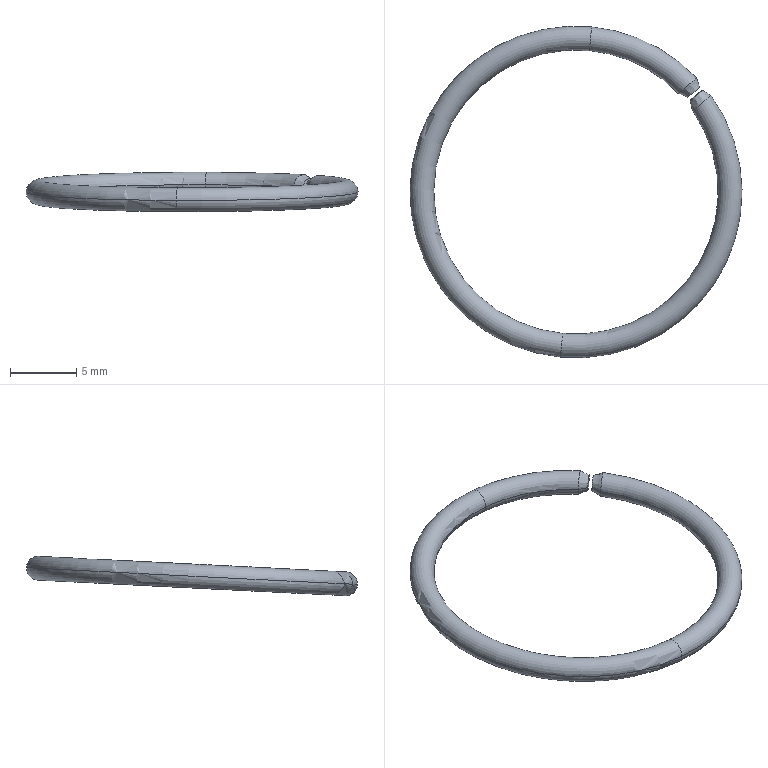Part | SolidWorks | features BaseBody 1 | 1 solid | 12 faces | box 25.1 x 25.07 x 2.979 mm | volume 184.393 mm3 | torus 6 | spline 4 | plane 2
STEP:
#1=CARTESIAN_POINT('',(1925.446,-674.153,857.254));
#2=VERTEX_POINT('',#1);
#3=CARTESIAN_POINT('',(1932.144,-677.358,857.099));
#4=VERTEX_POINT('',#3);
#5=CARTESIAN_POINT('',(1924.436,-684.842,856.711));
#6=DIRECTION('',(0.001134,0.05057,-0.9987));
#7=DIRECTION('',(0.9956,-0.09388,-0.003624));
#8=AXIS2_PLACEMENT_3D('',#5,#6,#7);
#9=CIRCLE('',#8,10.75);
#10=EDGE_CURVE('',#2,#4,#9,.T.);
#11=ORIENTED_EDGE('',*,*,#10,.F.);
#12=CARTESIAN_POINT('',(1925.615,-672.363,857.345));
#13=VERTEX_POINT('',#12);
#14=CARTESIAN_POINT('',(1925.531,-673.258,857.299));
#15=DIRECTION('',(0.9956,-0.09388,-0.003624));
#16=DIRECTION('',(0.09388,0.9956,0.));
#17=AXIS2_PLACEMENT_3D('',#14,#15,#16);
#18=CIRCLE('',#17,0.9);
#19=EDGE_CURVE('',#2,#13,#18,.T.);
#20=ORIENTED_EDGE('',*,*,#19,.T.);
#21=CARTESIAN_POINT('',(1933.534,-676.209,857.159));
#22=VERTEX_POINT('',#21);
#23=CARTESIAN_POINT('',(1924.436,-684.842,856.711));
#24=DIRECTION('',(-0.001134,-0.05057,0.9987));
#25=DIRECTION('',(0.9956,-0.09388,-0.003624));
#26=AXIS2_PLACEMENT_3D('',#23,#24,#25);
#27=CIRCLE('',#26,12.55);
#28=EDGE_CURVE('',#22,#13,#27,.T.);
#29=ORIENTED_EDGE('',*,*,#28,.F.);
#30=CARTESIAN_POINT('',(1932.144,-677.358,857.099));
#31=CARTESIAN_POINT('',(1932.144,-677.352,856.98));
#32=CARTESIAN_POINT('',(1932.162,-677.332,856.866));
#33=CARTESIAN_POINT('',(1932.232,-677.262,856.65));
#34=CARTESIAN_POINT('',(1932.283,-677.215,856.553));
#35=CARTESIAN_POINT('',(1932.411,-677.098,856.392));
#36=CARTESIAN_POINT('',(1932.488,-677.03,856.329));
#37=CARTESIAN_POINT('',(1932.657,-676.889,856.246));
#38=CARTESIAN_POINT('',(1932.748,-676.812,856.226));
#39=CARTESIAN_POINT('',(1932.928,-676.662,856.234));
#40=CARTESIAN_POINT('',(1933.02,-676.588,856.261));
#41=CARTESIAN_POINT('',(1933.187,-676.453,856.358));
#42=CARTESIAN_POINT('',(1933.264,-676.392,856.428));
#43=CARTESIAN_POINT('',(1933.459,-676.247,856.685));
#44=CARTESIAN_POINT('',(1933.534,-676.197,856.921));
#45=CARTESIAN_POINT('',(1933.534,-676.209,857.159));
#46=B_SPLINE_CURVE_WITH_KNOTS('',3,(#30,#31,#32,#33,#34,#35,#36,#37,#38,#39,#40,#41,#42,#43,#44,#45),.UNSPECIFIED.,.F.,.F.,(4,2,2,2,2,2,2,4),(0.,0.0003506,0.0007011,0.001052,0.001402,0.001753,0.002103,0.002805),.UNSPECIFIED.);
#47=EDGE_CURVE('',#4,#22,#46,.T.);
#48=ORIENTED_EDGE('',*,*,#47,.F.);
#49=EDGE_LOOP('',(#11,#20,#29,#48));
#50=FACE_OUTER_BOUND('',#49,.T.);
#51=CARTESIAN_POINT('',(1924.436,-684.842,856.711));
#52=DIRECTION('',(-0.001134,-0.05057,0.9987));
#53=DIRECTION('',(-0.09394,-0.9943,-0.05046));
#54=AXIS2_PLACEMENT_3D('',#51,#52,#53);
#55=TOROIDAL_SURFACE('',#54,11.65,0.9);
#56=ADVANCED_FACE('',(#50),#55,.T.);
#57=ORIENTED_EDGE('',*,*,#19,.F.);
#58=CARTESIAN_POINT('',(1923.426,-695.531,856.169));
#59=VERTEX_POINT('',#58);
#60=CARTESIAN_POINT('',(1924.436,-684.842,856.711));
#61=DIRECTION('',(0.001134,0.05057,-0.9987));
#62=DIRECTION('',(0.9956,-0.09388,-0.003624));
#63=AXIS2_PLACEMENT_3D('',#60,#61,#62);
#64=CIRCLE('',#63,10.75);
#65=EDGE_CURVE('',#59,#2,#64,.T.);
#66=ORIENTED_EDGE('',*,*,#65,.F.);
#67=CARTESIAN_POINT('',(1923.257,-697.32,856.078));
#68=VERTEX_POINT('',#67);
#69=CARTESIAN_POINT('',(1923.342,-696.425,856.124));
#70=DIRECTION('',(-0.9956,0.09388,0.003624));
#71=DIRECTION('',(-0.09388,-0.9956,0.));
#72=AXIS2_PLACEMENT_3D('',#69,#70,#71);
#73=CIRCLE('',#72,0.9);
#74=EDGE_CURVE('',#59,#68,#73,.T.);
#75=ORIENTED_EDGE('',*,*,#74,.T.);
#76=CARTESIAN_POINT('',(1924.436,-684.842,856.711));
#77=DIRECTION('',(-0.001134,-0.05057,0.9987));
#78=DIRECTION('',(0.9956,-0.09388,-0.003624));
#79=AXIS2_PLACEMENT_3D('',#76,#77,#78);
#80=CIRCLE('',#79,12.55);
#81=EDGE_CURVE('',#13,#68,#80,.T.);
#82=ORIENTED_EDGE('',*,*,#81,.F.);
#83=EDGE_LOOP('',(#57,#66,#75,#82));
#84=FACE_OUTER_BOUND('',#83,.T.);
#85=CARTESIAN_POINT('',(1924.436,-684.842,856.711));
#86=DIRECTION('',(-0.001134,-0.05057,0.9987));
#87=DIRECTION('',(-0.09394,-0.9943,-0.05046));
#88=AXIS2_PLACEMENT_3D('',#85,#86,#87);
#89=TOROIDAL_SURFACE('',#88,11.65,0.9);
#90=ADVANCED_FACE('',(#84),#89,.T.);
#91=ORIENTED_EDGE('',*,*,#28,.T.);
#92=CARTESIAN_POINT('',(1925.531,-673.258,857.299));
#93=DIRECTION('',(0.9956,-0.09388,-0.003624));
#94=DIRECTION('',(0.09388,0.9956,0.));
#95=AXIS2_PLACEMENT_3D('',#92,#93,#94);
#96=CIRCLE('',#95,0.9);
#97=EDGE_CURVE('',#13,#2,#96,.T.);
#98=ORIENTED_EDGE('',*,*,#97,.T.);
#99=ORIENTED_EDGE('',*,*,#10,.T.);
#100=CARTESIAN_POINT('',(1933.534,-676.209,857.159));
#101=CARTESIAN_POINT('',(1933.534,-676.215,857.278));
#102=CARTESIAN_POINT('',(1933.516,-676.235,857.392));
#103=CARTESIAN_POINT('',(1933.446,-676.304,857.608));
#104=CARTESIAN_POINT('',(1933.394,-676.351,857.705));
#105=CARTESIAN_POINT('',(1933.263,-676.464,857.866));
#106=CARTESIAN_POINT('',(1933.187,-676.532,857.93));
#107=CARTESIAN_POINT('',(1933.02,-676.676,858.012));
#108=CARTESIAN_POINT('',(1932.928,-676.752,858.032));
#109=CARTESIAN_POINT('',(1932.747,-676.902,858.024));
#110=CARTESIAN_POINT('',(1932.656,-676.976,857.997));
#111=CARTESIAN_POINT('',(1932.487,-677.109,857.9));
#112=CARTESIAN_POINT('',(1932.41,-677.17,857.831));
#113=CARTESIAN_POINT('',(1932.219,-677.32,857.573));
#114=CARTESIAN_POINT('',(1932.144,-677.37,857.337));
#115=CARTESIAN_POINT('',(1932.144,-677.358,857.099));
#116=B_SPLINE_CURVE_WITH_KNOTS('',3,(#100,#101,#102,#103,#104,#105,#106,#107,#108,#109,#110,#111,#112,#113,#114,#115),.UNSPECIFIED.,.F.,.F.,(4,2,2,2,2,2,2,4),(0.,0.0003506,0.0007012,0.001052,0.001402,0.001753,0.002104,0.002805),.UNSPECIFIED.);
#117=EDGE_CURVE('',#22,#4,#116,.T.);
#118=ORIENTED_EDGE('',*,*,#117,.F.);
#119=EDGE_LOOP('',(#91,#98,#99,#118));
#120=FACE_OUTER_BOUND('',#119,.T.);
#121=CARTESIAN_POINT('',(1924.436,-684.842,856.711));
#122=DIRECTION('',(-0.001134,-0.05057,0.9987));
#123=DIRECTION('',(-0.09394,-0.9943,-0.05046));
#124=AXIS2_PLACEMENT_3D('',#121,#122,#123);
#125=TOROIDAL_SURFACE('',#124,11.65,0.9);
#126=ADVANCED_FACE('',(#120),#125,.T.);
#127=ORIENTED_EDGE('',*,*,#97,.F.);
#128=ORIENTED_EDGE('',*,*,#81,.T.);
#129=CARTESIAN_POINT('',(1923.342,-696.425,856.124));
#130=DIRECTION('',(-0.9956,0.09388,0.003624));
#131=DIRECTION('',(-0.09388,-0.9956,0.));
#132=AXIS2_PLACEMENT_3D('',#129,#130,#131);
#133=CIRCLE('',#132,0.9);
#134=EDGE_CURVE('',#68,#59,#133,.T.);
#135=ORIENTED_EDGE('',*,*,#134,.T.);
#136=ORIENTED_EDGE('',*,*,#65,.T.);
#137=EDGE_LOOP('',(#127,#128,#135,#136));
#138=FACE_OUTER_BOUND('',#137,.T.);
#139=CARTESIAN_POINT('',(1924.436,-684.842,856.711));
#140=DIRECTION('',(-0.001134,-0.05057,0.9987));
#141=DIRECTION('',(-0.09394,-0.9943,-0.05046));
#142=AXIS2_PLACEMENT_3D('',#139,#140,#141);
#143=TOROIDAL_SURFACE('',#142,11.65,0.9);
#144=ADVANCED_FACE('',(#138),#143,.T.);
#145=ORIENTED_EDGE('',*,*,#134,.F.);
#146=CARTESIAN_POINT('',(1934.63,-677.531,857.093));
#147=VERTEX_POINT('',#146);
#148=CARTESIAN_POINT('',(1924.436,-684.842,856.711));
#149=DIRECTION('',(-0.001134,-0.05057,0.9987));
#150=DIRECTION('',(0.9956,-0.09388,-0.003624));
#151=AXIS2_PLACEMENT_3D('',#148,#149,#150);
#152=CIRCLE('',#151,12.55);
#153=EDGE_CURVE('',#68,#147,#152,.T.);
#154=ORIENTED_EDGE('',*,*,#153,.T.);
#155=CARTESIAN_POINT('',(1933.239,-678.68,857.033));
#156=VERTEX_POINT('',#155);
#157=CARTESIAN_POINT('',(1933.239,-678.68,857.033));
#158=CARTESIAN_POINT('',(1933.239,-678.686,857.152));
#159=CARTESIAN_POINT('',(1933.257,-678.678,857.268));
#160=CARTESIAN_POINT('',(1933.327,-678.631,857.49));
#161=CARTESIAN_POINT('',(1933.378,-678.594,857.592));
#162=CARTESIAN_POINT('',(1933.509,-678.498,857.764));
#163=CARTESIAN_POINT('',(1933.586,-678.437,857.834));
#164=CARTESIAN_POINT('',(1933.752,-678.302,857.931));
#165=CARTESIAN_POINT('',(1933.844,-678.228,857.958));
#166=CARTESIAN_POINT('',(1934.025,-678.079,857.966));
#167=CARTESIAN_POINT('',(1934.116,-678.001,857.947));
#168=CARTESIAN_POINT('',(1934.284,-677.859,857.864));
#169=CARTESIAN_POINT('',(1934.362,-677.792,857.801));
#170=CARTESIAN_POINT('',(1934.554,-677.618,857.56));
#171=CARTESIAN_POINT('',(1934.63,-677.544,857.331));
#172=CARTESIAN_POINT('',(1934.63,-677.531,857.093));
#173=B_SPLINE_CURVE_WITH_KNOTS('',3,(#157,#158,#159,#160,#161,#162,#163,#164,#165,#166,#167,#168,#169,#170,#171,#172),.UNSPECIFIED.,.F.,.F.,(4,2,2,2,2,2,2,4),(0.,0.0003506,0.0007011,0.001052,0.001402,0.001753,0.002103,0.002805),.UNSPECIFIED.);
#174=EDGE_CURVE('',#156,#147,#173,.T.);
#175=ORIENTED_EDGE('',*,*,#174,.F.);
#176=CARTESIAN_POINT('',(1924.436,-684.842,856.711));
#177=DIRECTION('',(0.001134,0.05057,-0.9987));
#178=DIRECTION('',(0.9956,-0.09388,-0.003624));
#179=AXIS2_PLACEMENT_3D('',#176,#177,#178);
#180=CIRCLE('',#179,10.75);
#181=EDGE_CURVE('',#156,#59,#180,.T.);
#182=ORIENTED_EDGE('',*,*,#181,.T.);
#183=EDGE_LOOP('',(#145,#154,#175,#182));
#184=FACE_OUTER_BOUND('',#183,.T.);
#185=CARTESIAN_POINT('',(1924.436,-684.842,856.711));
#186=DIRECTION('',(-0.001134,-0.05057,0.9987));
#187=DIRECTION('',(-0.09394,-0.9943,-0.05046));
#188=AXIS2_PLACEMENT_3D('',#185,#186,#187);
#189=TOROIDAL_SURFACE('',#188,11.65,0.9);
#190=ADVANCED_FACE('',(#184),#189,.T.);
#191=ORIENTED_EDGE('',*,*,#74,.F.);
#192=ORIENTED_EDGE('',*,*,#181,.F.);
#193=CARTESIAN_POINT('',(1934.63,-677.531,857.093));
#194=CARTESIAN_POINT('',(1934.63,-677.525,856.974));
#195=CARTESIAN_POINT('',(1934.613,-677.534,856.859));
#196=CARTESIAN_POINT('',(1934.543,-677.581,856.636));
#197=CARTESIAN_POINT('',(1934.492,-677.619,856.535));
#198=CARTESIAN_POINT('',(1934.365,-677.719,856.363));
#199=CARTESIAN_POINT('',(1934.287,-677.779,856.293));
#200=CARTESIAN_POINT('',(1934.119,-677.912,856.196));
#201=CARTESIAN_POINT('',(1934.028,-677.987,856.168));
#202=CARTESIAN_POINT('',(1933.847,-678.136,856.16));
#203=CARTESIAN_POINT('',(1933.755,-678.213,856.18));
#204=CARTESIAN_POINT('',(1933.589,-678.357,856.262));
#205=CARTESIAN_POINT('',(1933.511,-678.424,856.325));
#206=CARTESIAN_POINT('',(1933.315,-678.594,856.566));
#207=CARTESIAN_POINT('',(1933.24,-678.668,856.795));
#208=CARTESIAN_POINT('',(1933.239,-678.68,857.033));
#209=B_SPLINE_CURVE_WITH_KNOTS('',3,(#193,#194,#195,#196,#197,#198,#199,#200,#201,#202,#203,#204,#205,#206,#207,#208),.UNSPECIFIED.,.F.,.F.,(4,2,2,2,2,2,2,4),(0.,0.0003506,0.0007012,0.001052,0.001402,0.001753,0.002104,0.002805),.UNSPECIFIED.);
#210=EDGE_CURVE('',#147,#156,#209,.T.);
#211=ORIENTED_EDGE('',*,*,#210,.F.);
#212=ORIENTED_EDGE('',*,*,#153,.F.);
#213=EDGE_LOOP('',(#191,#192,#211,#212));
#214=FACE_OUTER_BOUND('',#213,.T.);
#215=CARTESIAN_POINT('',(1924.436,-684.842,856.711));
#216=DIRECTION('',(-0.001134,-0.05057,0.9987));
#217=DIRECTION('',(-0.09394,-0.9943,-0.05046));
#218=AXIS2_PLACEMENT_3D('',#215,#216,#217);
#219=TOROIDAL_SURFACE('',#218,11.65,0.9);
#220=ADVANCED_FACE('',(#214),#219,.T.);
#221=CARTESIAN_POINT('',(1933.785,-676.906,857.124));
#222=VERTEX_POINT('',#221);
#223=CARTESIAN_POINT('',(1933.534,-676.209,857.159));
#224=DIRECTION('',(-0.3381,0.9399,0.04721));
#225=VECTOR('',#224,1000.);
#226=LINE('',#223,#225);
#227=EDGE_CURVE('',#222,#22,#226,.T.);
#228=ORIENTED_EDGE('',*,*,#227,.F.);
#229=CARTESIAN_POINT('',(1932.863,-677.669,857.084));
#230=VERTEX_POINT('',#229);
#231=CARTESIAN_POINT('',(1932.863,-677.669,857.084));
#232=CARTESIAN_POINT('',(1932.863,-677.667,857.045));
#233=CARTESIAN_POINT('',(1932.872,-677.653,856.927));
#234=CARTESIAN_POINT('',(1932.942,-677.584,856.707));
#235=CARTESIAN_POINT('',(1933.146,-677.405,856.498));
#236=CARTESIAN_POINT('',(1933.454,-677.149,856.488));
#237=CARTESIAN_POINT('',(1933.688,-676.966,856.702));
#238=CARTESIAN_POINT('',(1933.774,-676.907,856.948));
#239=CARTESIAN_POINT('',(1933.785,-676.904,857.08));
#240=CARTESIAN_POINT('',(1933.785,-676.906,857.124));
#241=B_SPLINE_CURVE_WITH_KNOTS('',3,(#231,#232,#233,#234,#235,#236,#237,#238,#239,#240),.UNSPECIFIED.,.F.,.F.,(4,1,1,1,1,1,1,4),(0.,0.06667,0.2,0.4,0.6,0.8,0.9333,1.),.UNSPECIFIED.);
#242=EDGE_CURVE('',#230,#222,#241,.T.);
#243=ORIENTED_EDGE('',*,*,#242,.F.);
#244=CARTESIAN_POINT('',(1932.144,-677.358,857.099));
#245=DIRECTION('',(0.918,-0.3961,-0.01902));
#246=VECTOR('',#245,1000.);
#247=LINE('',#244,#246);
#248=EDGE_CURVE('',#4,#230,#247,.T.);
#249=ORIENTED_EDGE('',*,*,#248,.F.);
#250=ORIENTED_EDGE('',*,*,#47,.T.);
#251=EDGE_LOOP('',(#228,#243,#249,#250));
#252=FACE_OUTER_BOUND('',#251,.T.);
#253=CARTESIAN_POINT('',(1932.103,-677.341,857.17));
#254=CARTESIAN_POINT('',(1932.37,-677.457,857.154));
#255=CARTESIAN_POINT('',(1932.638,-677.572,857.138));
#256=CARTESIAN_POINT('',(1932.905,-677.687,857.123));
#257=CARTESIAN_POINT('',(1932.101,-677.341,857.146));
#258=CARTESIAN_POINT('',(1932.369,-677.457,857.134));
#259=CARTESIAN_POINT('',(1932.637,-677.572,857.122));
#260=CARTESIAN_POINT('',(1932.905,-677.687,857.11));
#261=CARTESIAN_POINT('',(1932.099,-677.339,857.056));
#262=CARTESIAN_POINT('',(1932.367,-677.455,857.057));
#263=CARTESIAN_POINT('',(1932.635,-677.57,857.058));
#264=CARTESIAN_POINT('',(1932.903,-677.686,857.059));
#265=CARTESIAN_POINT('',(1932.118,-677.312,856.833));
#266=CARTESIAN_POINT('',(1932.383,-677.432,856.866));
#267=CARTESIAN_POINT('',(1932.648,-677.552,856.899));
#268=CARTESIAN_POINT('',(1932.913,-677.672,856.932));
#269=CARTESIAN_POINT('',(1932.251,-677.182,856.47));
#270=CARTESIAN_POINT('',(1932.494,-677.324,856.553));
#271=CARTESIAN_POINT('',(1932.737,-677.465,856.636));
#272=CARTESIAN_POINT('',(1932.98,-677.606,856.719));
#273=CARTESIAN_POINT('',(1932.605,-676.873,856.178));
#274=CARTESIAN_POINT('',(1932.795,-677.06,856.29));
#275=CARTESIAN_POINT('',(1932.985,-677.247,856.403));
#276=CARTESIAN_POINT('',(1933.176,-677.434,856.515));
#277=CARTESIAN_POINT('',(1933.069,-676.491,856.224));
#278=CARTESIAN_POINT('',(1933.204,-676.722,856.317));
#279=CARTESIAN_POINT('',(1933.34,-676.954,856.409));
#280=CARTESIAN_POINT('',(1933.475,-677.185,856.502));
#281=CARTESIAN_POINT('',(1933.39,-676.243,856.56));
#282=CARTESIAN_POINT('',(1933.495,-676.497,856.61));
#283=CARTESIAN_POINT('',(1933.599,-676.751,856.659));
#284=CARTESIAN_POINT('',(1933.704,-677.005,856.709));
#285=CARTESIAN_POINT('',(1933.505,-676.166,856.912));
#286=CARTESIAN_POINT('',(1933.599,-676.426,856.925));
#287=CARTESIAN_POINT('',(1933.694,-676.687,856.937));
#288=CARTESIAN_POINT('',(1933.789,-676.947,856.95));
#289=CARTESIAN_POINT('',(1933.521,-676.163,857.121));
#290=CARTESIAN_POINT('',(1933.614,-676.424,857.112));
#291=CARTESIAN_POINT('',(1933.708,-676.684,857.103));
#292=CARTESIAN_POINT('',(1933.801,-676.944,857.094));
#293=CARTESIAN_POINT('',(1933.518,-676.169,857.204));
#294=CARTESIAN_POINT('',(1933.612,-676.429,857.186));
#295=CARTESIAN_POINT('',(1933.706,-676.689,857.169));
#296=CARTESIAN_POINT('',(1933.799,-676.948,857.152));
#297=CARTESIAN_POINT('',(1933.517,-676.171,857.225));
#298=CARTESIAN_POINT('',(1933.611,-676.431,857.206));
#299=CARTESIAN_POINT('',(1933.705,-676.69,857.186));
#300=CARTESIAN_POINT('',(1933.798,-676.95,857.166));
#301=B_SPLINE_SURFACE_WITH_KNOTS('',3,3,((#253,#254,#255,#256),(#257,#258,#259,#260),(#261,#262,#263,#264),(#265,#266,#267,#268),(#269,#270,#271,#272),(#273,#274,#275,#276),(#277,#278,#279,#280),(#281,#282,#283,#284),(#285,#286,#287,#288),(#289,#290,#291,#292),(#293,#294,#295,#296),(#297,#298,#299,#300)),.UNSPECIFIED.,.F.,.F.,.F.,(4,1,1,1,1,1,1,1,1,4),(4,4),(0.,0.02206,0.08578,0.2132,0.4044,0.5956,0.7868,0.9142,0.9779,1.),(0.,1.),.UNSPECIFIED.);
#302=ADVANCED_FACE('',(#252),#301,.T.);
#303=ORIENTED_EDGE('',*,*,#248,.T.);
#304=CARTESIAN_POINT('',(1933.785,-676.906,857.124));
#305=CARTESIAN_POINT('',(1933.785,-676.909,857.168));
#306=CARTESIAN_POINT('',(1933.774,-676.925,857.299));
#307=CARTESIAN_POINT('',(1933.687,-677.008,857.538));
#308=CARTESIAN_POINT('',(1933.452,-677.212,857.732));
#309=CARTESIAN_POINT('',(1933.145,-677.465,857.695));
#310=CARTESIAN_POINT('',(1932.941,-677.623,857.469));
#311=CARTESIAN_POINT('',(1932.872,-677.669,857.242));
#312=CARTESIAN_POINT('',(1932.863,-677.671,857.124));
#313=CARTESIAN_POINT('',(1932.863,-677.669,857.084));
#314=B_SPLINE_CURVE_WITH_KNOTS('',3,(#304,#305,#306,#307,#308,#309,#310,#311,#312,#313),.UNSPECIFIED.,.F.,.F.,(4,1,1,1,1,1,1,4),(0.,0.06667,0.2,0.4,0.6,0.8,0.9333,1.),.UNSPECIFIED.);
#315=EDGE_CURVE('',#222,#230,#314,.T.);
#316=ORIENTED_EDGE('',*,*,#315,.F.);
#317=ORIENTED_EDGE('',*,*,#227,.T.);
#318=ORIENTED_EDGE('',*,*,#117,.T.);
#319=EDGE_LOOP('',(#303,#316,#317,#318));
#320=FACE_OUTER_BOUND('',#319,.T.);
#321=CARTESIAN_POINT('',(1933.517,-676.165,857.097));
#322=CARTESIAN_POINT('',(1933.611,-676.425,857.09));
#323=CARTESIAN_POINT('',(1933.705,-676.685,857.084));
#324=CARTESIAN_POINT('',(1933.798,-676.945,857.077));
#325=CARTESIAN_POINT('',(1933.518,-676.165,857.118));
#326=CARTESIAN_POINT('',(1933.612,-676.425,857.109));
#327=CARTESIAN_POINT('',(1933.706,-676.685,857.101));
#328=CARTESIAN_POINT('',(1933.799,-676.945,857.092));
#329=CARTESIAN_POINT('',(1933.521,-676.167,857.202));
#330=CARTESIAN_POINT('',(1933.614,-676.427,857.184));
#331=CARTESIAN_POINT('',(1933.707,-676.687,857.167));
#332=CARTESIAN_POINT('',(1933.801,-676.947,857.15));
#333=CARTESIAN_POINT('',(1933.504,-676.191,857.409));
#334=CARTESIAN_POINT('',(1933.599,-676.449,857.37));
#335=CARTESIAN_POINT('',(1933.694,-676.707,857.332));
#336=CARTESIAN_POINT('',(1933.788,-676.964,857.293));
#337=CARTESIAN_POINT('',(1933.389,-676.303,857.751));
#338=CARTESIAN_POINT('',(1933.493,-676.551,857.676));
#339=CARTESIAN_POINT('',(1933.598,-676.799,857.601));
#340=CARTESIAN_POINT('',(1933.703,-677.047,857.526));
#341=CARTESIAN_POINT('',(1933.067,-676.584,858.06));
#342=CARTESIAN_POINT('',(1933.202,-676.805,857.944));
#343=CARTESIAN_POINT('',(1933.338,-677.025,857.829));
#344=CARTESIAN_POINT('',(1933.473,-677.246,857.714));
#345=CARTESIAN_POINT('',(1932.603,-676.969,858.066));
#346=CARTESIAN_POINT('',(1932.793,-677.143,857.935));
#347=CARTESIAN_POINT('',(1932.984,-677.318,857.805));
#348=CARTESIAN_POINT('',(1933.174,-677.492,857.675));
#349=CARTESIAN_POINT('',(1932.25,-677.247,857.743));
#350=CARTESIAN_POINT('',(1932.493,-677.379,857.647));
#351=CARTESIAN_POINT('',(1932.736,-677.511,857.55));
#352=CARTESIAN_POINT('',(1932.979,-677.643,857.454));
#353=CARTESIAN_POINT('',(1932.118,-677.339,857.368));
#354=CARTESIAN_POINT('',(1932.383,-677.455,857.324));
#355=CARTESIAN_POINT('',(1932.648,-677.571,857.28));
#356=CARTESIAN_POINT('',(1932.913,-677.687,857.235));
#357=CARTESIAN_POINT('',(1932.099,-677.343,857.144));
#358=CARTESIAN_POINT('',(1932.367,-677.458,857.132));
#359=CARTESIAN_POINT('',(1932.635,-677.573,857.12));
#360=CARTESIAN_POINT('',(1932.903,-677.688,857.108));
#361=CARTESIAN_POINT('',(1932.102,-677.337,857.054));
#362=CARTESIAN_POINT('',(1932.369,-677.453,857.055));
#363=CARTESIAN_POINT('',(1932.637,-677.569,857.056));
#364=CARTESIAN_POINT('',(1932.905,-677.685,857.057));
#365=CARTESIAN_POINT('',(1932.103,-677.334,857.031));
#366=CARTESIAN_POINT('',(1932.37,-677.451,857.035));
#367=CARTESIAN_POINT('',(1932.638,-677.567,857.04));
#368=CARTESIAN_POINT('',(1932.905,-677.684,857.044));
#369=B_SPLINE_SURFACE_WITH_KNOTS('',3,3,((#321,#322,#323,#324),(#325,#326,#327,#328),(#329,#330,#331,#332),(#333,#334,#335,#336),(#337,#338,#339,#340),(#341,#342,#343,#344),(#345,#346,#347,#348),(#349,#350,#351,#352),(#353,#354,#355,#356),(#357,#358,#359,#360),(#361,#362,#363,#364),(#365,#366,#367,#368)),.UNSPECIFIED.,.F.,.F.,.F.,(4,1,1,1,1,1,1,1,1,4),(4,4),(0.,0.02206,0.08578,0.2132,0.4044,0.5956,0.7868,0.9142,0.9779,1.),(0.,1.),.UNSPECIFIED.);
#370=ADVANCED_FACE('',(#320),#369,.T.);
#371=ORIENTED_EDGE('',*,*,#242,.T.);
#372=ORIENTED_EDGE('',*,*,#315,.T.);
#373=EDGE_LOOP('',(#371,#372));
#374=FACE_OUTER_BOUND('',#373,.T.);
#375=CARTESIAN_POINT('',(1924.335,-684.672,855.819));
#376=DIRECTION('',(-0.6376,0.7695,0.03824));
#377=DIRECTION('',(0.001134,0.05057,-0.9987));
#378=AXIS2_PLACEMENT_3D('',#375,#376,#377);
#379=PLANE('',#378);
#380=ADVANCED_FACE('',(#374),#379,.F.);
#381=CARTESIAN_POINT('',(1933.069,-677.917,857.072));
#382=VERTEX_POINT('',#381);
#383=CARTESIAN_POINT('',(1933.239,-678.68,857.033));
#384=DIRECTION('',(-0.2179,0.9747,0.04911));
#385=VECTOR('',#384,1000.);
#386=LINE('',#383,#385);
#387=EDGE_CURVE('',#156,#382,#386,.T.);
#388=ORIENTED_EDGE('',*,*,#387,.T.);
#389=CARTESIAN_POINT('',(1933.991,-677.155,857.112));
#390=VERTEX_POINT('',#389);
#391=CARTESIAN_POINT('',(1933.991,-677.155,857.112));
#392=CARTESIAN_POINT('',(1933.991,-677.152,857.068));
#393=CARTESIAN_POINT('',(1933.98,-677.155,856.935));
#394=CARTESIAN_POINT('',(1933.893,-677.214,856.689));
#395=CARTESIAN_POINT('',(1933.659,-677.397,856.475));
#396=CARTESIAN_POINT('',(1933.352,-677.653,856.485));
#397=CARTESIAN_POINT('',(1933.148,-677.832,856.694));
#398=CARTESIAN_POINT('',(1933.078,-677.901,856.915));
#399=CARTESIAN_POINT('',(1933.069,-677.915,857.032));
#400=CARTESIAN_POINT('',(1933.069,-677.917,857.072));
#401=B_SPLINE_CURVE_WITH_KNOTS('',3,(#391,#392,#393,#394,#395,#396,#397,#398,#399,#400),.UNSPECIFIED.,.F.,.F.,(4,1,1,1,1,1,1,4),(0.,0.06667,0.2,0.4,0.6,0.8,0.9333,1.),.UNSPECIFIED.);
#402=EDGE_CURVE('',#390,#382,#401,.T.);
#403=ORIENTED_EDGE('',*,*,#402,.F.);
#404=CARTESIAN_POINT('',(1934.63,-677.531,857.093));
#405=DIRECTION('',(0.8612,-0.5076,-0.02473));
#406=VECTOR('',#405,1000.);
#407=LINE('',#404,#406);
#408=EDGE_CURVE('',#390,#147,#407,.T.);
#409=ORIENTED_EDGE('',*,*,#408,.T.);
#410=ORIENTED_EDGE('',*,*,#210,.T.);
#411=EDGE_LOOP('',(#388,#403,#409,#410));
#412=FACE_OUTER_BOUND('',#411,.T.);
#413=CARTESIAN_POINT('',(1933.252,-678.728,857.1));
#414=CARTESIAN_POINT('',(1933.188,-678.443,857.104));
#415=CARTESIAN_POINT('',(1933.124,-678.159,857.109));
#416=CARTESIAN_POINT('',(1933.06,-677.874,857.113));
#417=CARTESIAN_POINT('',(1933.25,-678.728,857.077));
#418=CARTESIAN_POINT('',(1933.187,-678.443,857.085));
#419=CARTESIAN_POINT('',(1933.123,-678.159,857.092));
#420=CARTESIAN_POINT('',(1933.059,-677.874,857.1));
#421=CARTESIAN_POINT('',(1933.248,-678.725,856.987));
#422=CARTESIAN_POINT('',(1933.184,-678.441,857.008));
#423=CARTESIAN_POINT('',(1933.121,-678.157,857.028));
#424=CARTESIAN_POINT('',(1933.058,-677.872,857.049));
#425=CARTESIAN_POINT('',(1933.267,-678.698,856.764));
#426=CARTESIAN_POINT('',(1933.201,-678.418,856.817));
#427=CARTESIAN_POINT('',(1933.134,-678.138,856.87));
#428=CARTESIAN_POINT('',(1933.068,-677.858,856.923));
#429=CARTESIAN_POINT('',(1933.401,-678.571,856.401));
#430=CARTESIAN_POINT('',(1933.312,-678.311,856.504));
#431=CARTESIAN_POINT('',(1933.223,-678.052,856.607));
#432=CARTESIAN_POINT('',(1933.134,-677.792,856.71));
#433=CARTESIAN_POINT('',(1933.757,-678.263,856.109));
#434=CARTESIAN_POINT('',(1933.614,-678.049,856.241));
#435=CARTESIAN_POINT('',(1933.472,-677.834,856.373));
#436=CARTESIAN_POINT('',(1933.33,-677.62,856.506));
#437=CARTESIAN_POINT('',(1934.221,-677.881,856.155));
#438=CARTESIAN_POINT('',(1934.024,-677.711,856.267));
#439=CARTESIAN_POINT('',(1933.826,-677.541,856.38));
#440=CARTESIAN_POINT('',(1933.629,-677.371,856.493));
#441=CARTESIAN_POINT('',(1934.54,-677.631,856.491));
#442=CARTESIAN_POINT('',(1934.313,-677.485,856.561));
#443=CARTESIAN_POINT('',(1934.086,-677.338,856.63));
#444=CARTESIAN_POINT('',(1933.858,-677.192,856.7));
#445=CARTESIAN_POINT('',(1934.654,-677.554,856.843));
#446=CARTESIAN_POINT('',(1934.417,-677.414,856.876));
#447=CARTESIAN_POINT('',(1934.18,-677.273,856.908));
#448=CARTESIAN_POINT('',(1933.943,-677.133,856.94));
#449=CARTESIAN_POINT('',(1934.67,-677.551,857.051));
#450=CARTESIAN_POINT('',(1934.432,-677.411,857.062));
#451=CARTESIAN_POINT('',(1934.194,-677.271,857.073));
#452=CARTESIAN_POINT('',(1933.955,-677.13,857.084));
#453=CARTESIAN_POINT('',(1934.668,-677.557,857.135));
#454=CARTESIAN_POINT('',(1934.43,-677.416,857.137));
#455=CARTESIAN_POINT('',(1934.192,-677.275,857.14));
#456=CARTESIAN_POINT('',(1933.954,-677.135,857.142));
#457=CARTESIAN_POINT('',(1934.667,-677.559,857.156));
#458=CARTESIAN_POINT('',(1934.429,-677.418,857.156));
#459=CARTESIAN_POINT('',(1934.191,-677.277,857.156));
#460=CARTESIAN_POINT('',(1933.953,-677.136,857.157));
#461=B_SPLINE_SURFACE_WITH_KNOTS('',3,3,((#413,#414,#415,#416),(#417,#418,#419,#420),(#421,#422,#423,#424),(#425,#426,#427,#428),(#429,#430,#431,#432),(#433,#434,#435,#436),(#437,#438,#439,#440),(#441,#442,#443,#444),(#445,#446,#447,#448),(#449,#450,#451,#452),(#453,#454,#455,#456),(#457,#458,#459,#460)),.UNSPECIFIED.,.F.,.F.,.F.,(4,1,1,1,1,1,1,1,1,4),(4,4),(0.,0.02189,0.08564,0.2131,0.4044,0.5956,0.7869,0.9144,0.9781,1.),(0.,1.),.UNSPECIFIED.);
#462=ADVANCED_FACE('',(#412),#461,.F.);
#463=ORIENTED_EDGE('',*,*,#408,.F.);
#464=CARTESIAN_POINT('',(1933.069,-677.917,857.072));
#465=CARTESIAN_POINT('',(1933.069,-677.919,857.111));
#466=CARTESIAN_POINT('',(1933.077,-677.917,857.23));
#467=CARTESIAN_POINT('',(1933.147,-677.871,857.456));
#468=CARTESIAN_POINT('',(1933.351,-677.713,857.683));
#469=CARTESIAN_POINT('',(1933.658,-677.46,857.719));
#470=CARTESIAN_POINT('',(1933.892,-677.257,857.525));
#471=CARTESIAN_POINT('',(1933.979,-677.173,857.287));
#472=CARTESIAN_POINT('',(1933.991,-677.157,857.155));
#473=CARTESIAN_POINT('',(1933.991,-677.155,857.112));
#474=B_SPLINE_CURVE_WITH_KNOTS('',3,(#464,#465,#466,#467,#468,#469,#470,#471,#472,#473),.UNSPECIFIED.,.F.,.F.,(4,1,1,1,1,1,1,4),(0.,0.06667,0.2,0.4,0.6,0.8,0.9333,1.),.UNSPECIFIED.);
#475=EDGE_CURVE('',#382,#390,#474,.T.);
#476=ORIENTED_EDGE('',*,*,#475,.F.);
#477=ORIENTED_EDGE('',*,*,#387,.F.);
#478=ORIENTED_EDGE('',*,*,#174,.T.);
#479=EDGE_LOOP('',(#463,#476,#477,#478));
#480=FACE_OUTER_BOUND('',#479,.T.);
#481=CARTESIAN_POINT('',(1934.667,-677.552,857.028));
#482=CARTESIAN_POINT('',(1934.429,-677.412,857.042));
#483=CARTESIAN_POINT('',(1934.191,-677.272,857.055));
#484=CARTESIAN_POINT('',(1933.953,-677.132,857.068));
#485=CARTESIAN_POINT('',(1934.668,-677.552,857.049));
#486=CARTESIAN_POINT('',(1934.43,-677.412,857.061));
#487=CARTESIAN_POINT('',(1934.192,-677.272,857.072));
#488=CARTESIAN_POINT('',(1933.954,-677.132,857.083));
#489=CARTESIAN_POINT('',(1934.67,-677.555,857.133));
#490=CARTESIAN_POINT('',(1934.432,-677.414,857.136));
#491=CARTESIAN_POINT('',(1934.194,-677.274,857.138));
#492=CARTESIAN_POINT('',(1933.955,-677.133,857.141));
#493=CARTESIAN_POINT('',(1934.654,-677.579,857.34));
#494=CARTESIAN_POINT('',(1934.417,-677.436,857.321));
#495=CARTESIAN_POINT('',(1934.18,-677.293,857.302));
#496=CARTESIAN_POINT('',(1933.943,-677.151,857.284));
#497=CARTESIAN_POINT('',(1934.539,-677.692,857.682));
#498=CARTESIAN_POINT('',(1934.312,-677.539,857.627));
#499=CARTESIAN_POINT('',(1934.085,-677.386,857.572));
#500=CARTESIAN_POINT('',(1933.857,-677.233,857.517));
#501=CARTESIAN_POINT('',(1934.219,-677.974,857.991));
#502=CARTESIAN_POINT('',(1934.022,-677.793,857.895));
#503=CARTESIAN_POINT('',(1933.825,-677.613,857.8));
#504=CARTESIAN_POINT('',(1933.628,-677.433,857.704));
#505=CARTESIAN_POINT('',(1933.755,-678.359,857.997));
#506=CARTESIAN_POINT('',(1933.613,-678.132,857.886));
#507=CARTESIAN_POINT('',(1933.471,-677.905,857.776));
#508=CARTESIAN_POINT('',(1933.329,-677.678,857.666));
#509=CARTESIAN_POINT('',(1933.4,-678.635,857.674));
#510=CARTESIAN_POINT('',(1933.311,-678.366,857.597));
#511=CARTESIAN_POINT('',(1933.222,-678.098,857.521));
#512=CARTESIAN_POINT('',(1933.133,-677.829,857.445));
#513=CARTESIAN_POINT('',(1933.266,-678.726,857.3));
#514=CARTESIAN_POINT('',(1933.2,-678.442,857.275));
#515=CARTESIAN_POINT('',(1933.134,-678.157,857.251));
#516=CARTESIAN_POINT('',(1933.067,-677.873,857.226));
#517=CARTESIAN_POINT('',(1933.248,-678.73,857.075));
#518=CARTESIAN_POINT('',(1933.184,-678.445,857.083));
#519=CARTESIAN_POINT('',(1933.121,-678.16,857.091));
#520=CARTESIAN_POINT('',(1933.058,-677.875,857.099));
#521=CARTESIAN_POINT('',(1933.25,-678.723,856.985));
#522=CARTESIAN_POINT('',(1933.187,-678.439,857.006));
#523=CARTESIAN_POINT('',(1933.123,-678.155,857.027));
#524=CARTESIAN_POINT('',(1933.059,-677.871,857.048));
#525=CARTESIAN_POINT('',(1933.252,-678.721,856.962));
#526=CARTESIAN_POINT('',(1933.188,-678.437,856.987));
#527=CARTESIAN_POINT('',(1933.124,-678.154,857.011));
#528=CARTESIAN_POINT('',(1933.06,-677.87,857.035));
#529=B_SPLINE_SURFACE_WITH_KNOTS('',3,3,((#481,#482,#483,#484),(#485,#486,#487,#488),(#489,#490,#491,#492),(#493,#494,#495,#496),(#497,#498,#499,#500),(#501,#502,#503,#504),(#505,#506,#507,#508),(#509,#510,#511,#512),(#513,#514,#515,#516),(#517,#518,#519,#520),(#521,#522,#523,#524),(#525,#526,#527,#528)),.UNSPECIFIED.,.F.,.F.,.F.,(4,1,1,1,1,1,1,1,1,4),(4,4),(0.,0.02189,0.08564,0.2131,0.4044,0.5956,0.7869,0.9144,0.9781,1.),(0.,1.),.UNSPECIFIED.);
#530=ADVANCED_FACE('',(#480),#529,.F.);
#531=ORIENTED_EDGE('',*,*,#402,.T.);
#532=ORIENTED_EDGE('',*,*,#475,.T.);
#533=EDGE_LOOP('',(#531,#532));
#534=FACE_OUTER_BOUND('',#533,.T.);
#535=CARTESIAN_POINT('',(1924.538,-685.011,857.604));
#536=DIRECTION('',(0.6376,-0.7695,-0.03824));
#537=DIRECTION('',(-0.001134,-0.05057,0.9987));
#538=AXIS2_PLACEMENT_3D('',#535,#536,#537);
#539=PLANE('',#538);
#540=ADVANCED_FACE('',(#534),#539,.F.);
#541=CLOSED_SHELL('',(#56,#90,#126,#144,#190,#220,#302,#370,#380,#462,#530,#540));
#542=MANIFOLD_SOLID_BREP('',#541);
#543=CARTESIAN_POINT('',(0.,0.,0.));
#544=DIRECTION('',(0.,0.,1.));
#545=DIRECTION('',(1.,0.,0.));
#546=AXIS2_PLACEMENT_3D('',#543,#544,#545);
#547=(LENGTH_UNIT()NAMED_UNIT(*)SI_UNIT(.MILLI.,.METRE.));
#548=UNCERTAINTY_MEASURE_WITH_UNIT(LENGTH_MEASURE(0.00001),#547,'','');
#549=(NAMED_UNIT(*)PLANE_ANGLE_UNIT()SI_UNIT($,.RADIAN.));
#550=(NAMED_UNIT(*)SI_UNIT($,.STERADIAN.)SOLID_ANGLE_UNIT());
#551=(GEOMETRIC_REPRESENTATION_CONTEXT(3)GLOBAL_UNCERTAINTY_ASSIGNED_CONTEXT((#548))GLOBAL_UNIT_ASSIGNED_CONTEXT((#547,#549,#550))REPRESENTATION_CONTEXT('',''));
#552=ADVANCED_BREP_SHAPE_REPRESENTATION('',(#542,#546),#551);